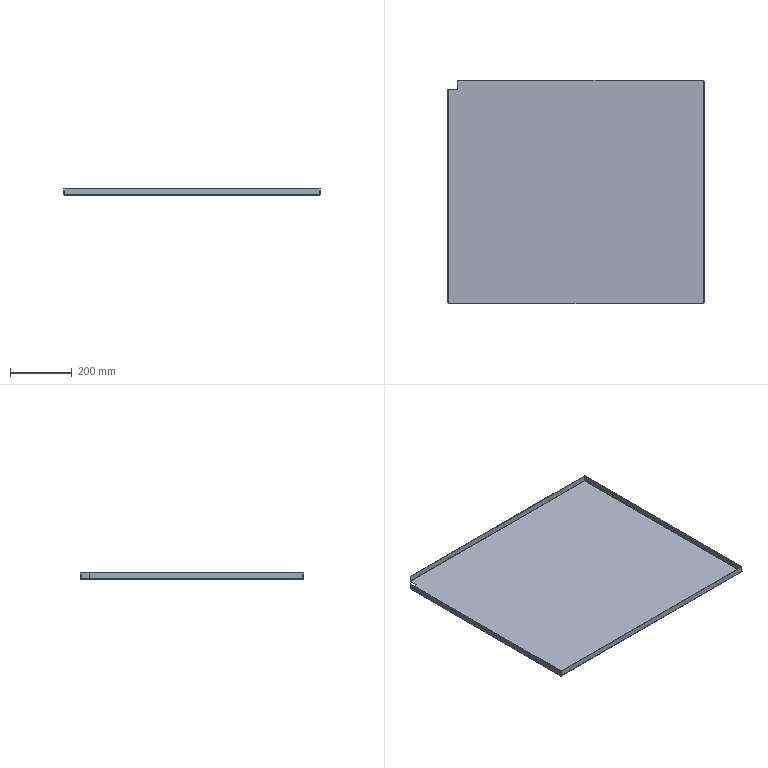Part | SolidWorks | 1 solid | 40 faces | box 830.001 x 723.001 x 20 mm | volume 981196 mm3 | plane 26 | cylinder 8 | spline 6 | commonest cylinder face diameters 0.2 x4 3.2 x4
STEP:
#1=CARTESIAN_POINT('',(-413.5,331.5,18.5));
#2=VERTEX_POINT('',#1);
#3=CARTESIAN_POINT('',(-413.5,331.5,0.1));
#4=VERTEX_POINT('',#3);
#5=CARTESIAN_POINT('',(-413.5,331.5,0.));
#6=DIRECTION('',(0.,0.,-1.));
#7=VECTOR('',#6,1000.);
#8=LINE('',#5,#7);
#9=EDGE_CURVE('',#2,#4,#8,.T.);
#10=ORIENTED_EDGE('',*,*,#9,.T.);
#11=CARTESIAN_POINT('',(-415.,331.5,0.1));
#12=VERTEX_POINT('',#11);
#13=CARTESIAN_POINT('',(-413.5,331.5,0.1));
#14=DIRECTION('',(-1.,0.,0.));
#15=VECTOR('',#14,1000.);
#16=LINE('',#13,#15);
#17=EDGE_CURVE('',#4,#12,#16,.T.);
#18=ORIENTED_EDGE('',*,*,#17,.T.);
#19=CARTESIAN_POINT('',(-415.,331.5,18.5));
#20=VERTEX_POINT('',#19);
#21=CARTESIAN_POINT('',(-415.,331.5,0.));
#22=DIRECTION('',(0.,0.,-1.));
#23=VECTOR('',#22,1000.);
#24=LINE('',#21,#23);
#25=EDGE_CURVE('',#20,#12,#24,.T.);
#26=ORIENTED_EDGE('',*,*,#25,.F.);
#27=CARTESIAN_POINT('',(-434.,331.5,18.5));
#28=DIRECTION('',(1.,0.,0.));
#29=VECTOR('',#28,1000.);
#30=LINE('',#27,#29);
#31=EDGE_CURVE('',#20,#2,#30,.T.);
#32=ORIENTED_EDGE('',*,*,#31,.T.);
#33=EDGE_LOOP('',(#10,#18,#26,#32));
#34=FACE_OUTER_BOUND('',#33,.T.);
#35=CARTESIAN_POINT('',(-434.,331.5,-1.5));
#36=DIRECTION('',(0.,-1.,0.));
#37=DIRECTION('',(0.,0.,-1.));
#38=AXIS2_PLACEMENT_3D('',#35,#36,#37);
#39=PLANE('',#38);
#40=ADVANCED_FACE('',(#34),#39,.F.);
#41=CARTESIAN_POINT('',(-413.4,331.5,-1.5));
#42=VERTEX_POINT('',#41);
#43=CARTESIAN_POINT('',(-384.,331.5,-1.5));
#44=VERTEX_POINT('',#43);
#45=CARTESIAN_POINT('',(-434.,331.5,-1.5));
#46=DIRECTION('',(1.,0.,0.));
#47=VECTOR('',#46,1000.);
#48=LINE('',#45,#47);
#49=EDGE_CURVE('',#42,#44,#48,.T.);
#50=ORIENTED_EDGE('',*,*,#49,.F.);
#51=CARTESIAN_POINT('',(-413.4,331.5,0.));
#52=VERTEX_POINT('',#51);
#53=CARTESIAN_POINT('',(-413.4,331.5,-1.5));
#54=DIRECTION('',(0.,0.,1.));
#55=VECTOR('',#54,1000.);
#56=LINE('',#53,#55);
#57=EDGE_CURVE('',#42,#52,#56,.T.);
#58=ORIENTED_EDGE('',*,*,#57,.T.);
#59=CARTESIAN_POINT('',(-384.,331.5,0.));
#60=VERTEX_POINT('',#59);
#61=CARTESIAN_POINT('',(0.,331.5,0.));
#62=DIRECTION('',(1.,0.,0.));
#63=VECTOR('',#62,1000.);
#64=LINE('',#61,#63);
#65=EDGE_CURVE('',#52,#60,#64,.T.);
#66=ORIENTED_EDGE('',*,*,#65,.T.);
#67=CARTESIAN_POINT('',(-384.,331.5,-1.5));
#68=DIRECTION('',(0.,0.,1.));
#69=VECTOR('',#68,1000.);
#70=LINE('',#67,#69);
#71=EDGE_CURVE('',#44,#60,#70,.T.);
#72=ORIENTED_EDGE('',*,*,#71,.F.);
#73=EDGE_LOOP('',(#50,#58,#66,#72));
#74=FACE_OUTER_BOUND('',#73,.T.);
#75=CARTESIAN_POINT('',(-434.,331.5,-1.5));
#76=DIRECTION('',(0.,-1.,0.));
#77=DIRECTION('',(0.,0.,-1.));
#78=AXIS2_PLACEMENT_3D('',#75,#76,#77);
#79=PLANE('',#78);
#80=ADVANCED_FACE('',(#74),#79,.F.);
#81=CARTESIAN_POINT('',(-384.,359.9,0.));
#82=VERTEX_POINT('',#81);
#83=CARTESIAN_POINT('',(-384.,0.,0.));
#84=DIRECTION('',(0.,1.,0.));
#85=VECTOR('',#84,1000.);
#86=LINE('',#83,#85);
#87=EDGE_CURVE('',#60,#82,#86,.T.);
#88=ORIENTED_EDGE('',*,*,#87,.T.);
#89=CARTESIAN_POINT('',(-384.,359.9,-1.5));
#90=VERTEX_POINT('',#89);
#91=CARTESIAN_POINT('',(-384.,359.9,0.));
#92=DIRECTION('',(0.,0.,-1.));
#93=VECTOR('',#92,1000.);
#94=LINE('',#91,#93);
#95=EDGE_CURVE('',#82,#90,#94,.T.);
#96=ORIENTED_EDGE('',*,*,#95,.T.);
#97=CARTESIAN_POINT('',(-384.,381.5,-1.5));
#98=DIRECTION('',(0.,1.,0.));
#99=VECTOR('',#98,1000.);
#100=LINE('',#97,#99);
#101=EDGE_CURVE('',#44,#90,#100,.T.);
#102=ORIENTED_EDGE('',*,*,#101,.F.);
#103=ORIENTED_EDGE('',*,*,#71,.T.);
#104=EDGE_LOOP('',(#88,#96,#102,#103));
#105=FACE_OUTER_BOUND('',#104,.T.);
#106=CARTESIAN_POINT('',(-384.,381.5,-1.5));
#107=DIRECTION('',(1.,0.,0.));
#108=DIRECTION('',(0.,0.,-1.));
#109=AXIS2_PLACEMENT_3D('',#106,#107,#108);
#110=PLANE('',#109);
#111=ADVANCED_FACE('',(#105),#110,.F.);
#112=CARTESIAN_POINT('',(-384.,361.5,0.1));
#113=VERTEX_POINT('',#112);
#114=CARTESIAN_POINT('',(-384.,361.5,18.5));
#115=VERTEX_POINT('',#114);
#116=CARTESIAN_POINT('',(-384.,361.5,0.));
#117=DIRECTION('',(0.,0.,1.));
#118=VECTOR('',#117,1000.);
#119=LINE('',#116,#118);
#120=EDGE_CURVE('',#113,#115,#119,.T.);
#121=ORIENTED_EDGE('',*,*,#120,.F.);
#122=CARTESIAN_POINT('',(-384.,360.,0.1));
#123=VERTEX_POINT('',#122);
#124=CARTESIAN_POINT('',(-384.,361.5,0.1));
#125=DIRECTION('',(0.,-1.,0.));
#126=VECTOR('',#125,1000.);
#127=LINE('',#124,#126);
#128=EDGE_CURVE('',#113,#123,#127,.T.);
#129=ORIENTED_EDGE('',*,*,#128,.T.);
#130=CARTESIAN_POINT('',(-384.,360.,18.5));
#131=VERTEX_POINT('',#130);
#132=CARTESIAN_POINT('',(-384.,360.,0.));
#133=DIRECTION('',(0.,0.,1.));
#134=VECTOR('',#133,1000.);
#135=LINE('',#132,#134);
#136=EDGE_CURVE('',#123,#131,#135,.T.);
#137=ORIENTED_EDGE('',*,*,#136,.T.);
#138=CARTESIAN_POINT('',(-384.,381.5,18.5));
#139=DIRECTION('',(0.,1.,0.));
#140=VECTOR('',#139,1000.);
#141=LINE('',#138,#140);
#142=EDGE_CURVE('',#131,#115,#141,.T.);
#143=ORIENTED_EDGE('',*,*,#142,.T.);
#144=EDGE_LOOP('',(#121,#129,#137,#143));
#145=FACE_OUTER_BOUND('',#144,.T.);
#146=CARTESIAN_POINT('',(-384.,381.5,-1.5));
#147=DIRECTION('',(1.,0.,0.));
#148=DIRECTION('',(0.,0.,-1.));
#149=AXIS2_PLACEMENT_3D('',#146,#147,#148);
#150=PLANE('',#149);
#151=ADVANCED_FACE('',(#145),#150,.F.);
#152=ORIENTED_EDGE('',*,*,#49,.T.);
#153=ORIENTED_EDGE('',*,*,#101,.T.);
#154=CARTESIAN_POINT('',(413.4,359.9,-1.5));
#155=VERTEX_POINT('',#154);
#156=CARTESIAN_POINT('',(-413.4,359.9,-1.5));
#157=DIRECTION('',(1.,0.,0.));
#158=VECTOR('',#157,1000.);
#159=LINE('',#156,#158);
#160=EDGE_CURVE('',#90,#155,#159,.T.);
#161=ORIENTED_EDGE('',*,*,#160,.T.);
#162=CARTESIAN_POINT('',(413.4,-359.9,-1.5));
#163=VERTEX_POINT('',#162);
#164=CARTESIAN_POINT('',(413.4,359.9,-1.5));
#165=DIRECTION('',(0.,-1.,0.));
#166=VECTOR('',#165,1000.);
#167=LINE('',#164,#166);
#168=EDGE_CURVE('',#155,#163,#167,.T.);
#169=ORIENTED_EDGE('',*,*,#168,.T.);
#170=CARTESIAN_POINT('',(-413.4,-359.9,-1.5));
#171=VERTEX_POINT('',#170);
#172=CARTESIAN_POINT('',(413.4,-359.9,-1.5));
#173=DIRECTION('',(-1.,0.,0.));
#174=VECTOR('',#173,1000.);
#175=LINE('',#172,#174);
#176=EDGE_CURVE('',#163,#171,#175,.T.);
#177=ORIENTED_EDGE('',*,*,#176,.T.);
#178=CARTESIAN_POINT('',(-413.4,-359.9,-1.5));
#179=DIRECTION('',(0.,1.,0.));
#180=VECTOR('',#179,1000.);
#181=LINE('',#178,#180);
#182=EDGE_CURVE('',#171,#42,#181,.T.);
#183=ORIENTED_EDGE('',*,*,#182,.T.);
#184=EDGE_LOOP('',(#152,#153,#161,#169,#177,#183));
#185=FACE_OUTER_BOUND('',#184,.T.);
#186=CARTESIAN_POINT('',(0.,0.,-1.5));
#187=DIRECTION('',(0.,0.,1.));
#188=DIRECTION('',(1.,0.,0.));
#189=AXIS2_PLACEMENT_3D('',#186,#187,#188);
#190=PLANE('',#189);
#191=ADVANCED_FACE('',(#185),#190,.F.);
#192=ORIENTED_EDGE('',*,*,#87,.F.);
#193=ORIENTED_EDGE('',*,*,#65,.F.);
#194=CARTESIAN_POINT('',(-413.4,-359.9,0.));
#195=VERTEX_POINT('',#194);
#196=CARTESIAN_POINT('',(-413.4,-359.9,0.));
#197=DIRECTION('',(0.,1.,0.));
#198=VECTOR('',#197,1000.);
#199=LINE('',#196,#198);
#200=EDGE_CURVE('',#195,#52,#199,.T.);
#201=ORIENTED_EDGE('',*,*,#200,.F.);
#202=CARTESIAN_POINT('',(413.4,-359.9,0.));
#203=VERTEX_POINT('',#202);
#204=CARTESIAN_POINT('',(413.4,-359.9,0.));
#205=DIRECTION('',(-1.,0.,0.));
#206=VECTOR('',#205,1000.);
#207=LINE('',#204,#206);
#208=EDGE_CURVE('',#203,#195,#207,.T.);
#209=ORIENTED_EDGE('',*,*,#208,.F.);
#210=CARTESIAN_POINT('',(413.4,359.9,0.));
#211=VERTEX_POINT('',#210);
#212=CARTESIAN_POINT('',(413.4,359.9,0.));
#213=DIRECTION('',(0.,-1.,0.));
#214=VECTOR('',#213,1000.);
#215=LINE('',#212,#214);
#216=EDGE_CURVE('',#211,#203,#215,.T.);
#217=ORIENTED_EDGE('',*,*,#216,.F.);
#218=CARTESIAN_POINT('',(-413.4,359.9,0.));
#219=DIRECTION('',(1.,0.,0.));
#220=VECTOR('',#219,1000.);
#221=LINE('',#218,#220);
#222=EDGE_CURVE('',#82,#211,#221,.T.);
#223=ORIENTED_EDGE('',*,*,#222,.F.);
#224=EDGE_LOOP('',(#192,#193,#201,#209,#217,#223));
#225=FACE_OUTER_BOUND('',#224,.T.);
#226=CARTESIAN_POINT('',(0.,0.,0.));
#227=DIRECTION('',(0.,0.,1.));
#228=DIRECTION('',(1.,0.,0.));
#229=AXIS2_PLACEMENT_3D('',#226,#227,#228);
#230=PLANE('',#229);
#231=ADVANCED_FACE('',(#225),#230,.T.);
#232=CARTESIAN_POINT('',(-413.5,-359.293,0.1));
#233=VERTEX_POINT('',#232);
#234=CARTESIAN_POINT('',(-413.5,-359.293,0.1));
#235=CARTESIAN_POINT('',(-413.5,-359.394,0.07382));
#236=CARTESIAN_POINT('',(-413.489,-359.495,0.0478));
#237=CARTESIAN_POINT('',(-413.452,-359.698,0.01078));
#238=CARTESIAN_POINT('',(-413.426,-359.799,0.));
#239=CARTESIAN_POINT('',(-413.4,-359.9,0.));
#240=B_SPLINE_CURVE_WITH_KNOTS('',3,(#234,#235,#236,#237,#238,#239),.UNSPECIFIED.,.F.,.F.,(4,2,4),(0.,0.5,1.),.UNSPECIFIED.);
#241=EDGE_CURVE('',#233,#195,#240,.T.);
#242=ORIENTED_EDGE('',*,*,#241,.F.);
#243=CARTESIAN_POINT('',(-415.,-359.293,0.1));
#244=VERTEX_POINT('',#243);
#245=CARTESIAN_POINT('',(-413.5,-359.293,0.1));
#246=DIRECTION('',(1.,0.,0.));
#247=VECTOR('',#246,1000.);
#248=LINE('',#245,#247);
#249=EDGE_CURVE('',#244,#233,#248,.T.);
#250=ORIENTED_EDGE('',*,*,#249,.F.);
#251=CARTESIAN_POINT('',(-415.,-359.293,0.1));
#252=CARTESIAN_POINT('',(-415.,-359.344,-0.1115));
#253=CARTESIAN_POINT('',(-414.96,-359.393,-0.3151));
#254=CARTESIAN_POINT('',(-414.799,-359.495,-0.7048));
#255=CARTESIAN_POINT('',(-414.681,-359.545,-0.881));
#256=CARTESIAN_POINT('',(-414.458,-359.621,-1.105));
#257=CARTESIAN_POINT('',(-414.378,-359.647,-1.171));
#258=CARTESIAN_POINT('',(-414.204,-359.697,-1.287));
#259=CARTESIAN_POINT('',(-414.11,-359.723,-1.338));
#260=CARTESIAN_POINT('',(-413.82,-359.799,-1.458));
#261=CARTESIAN_POINT('',(-413.612,-359.849,-1.5));
#262=CARTESIAN_POINT('',(-413.4,-359.9,-1.5));
#263=B_SPLINE_CURVE_WITH_KNOTS('',3,(#251,#252,#253,#254,#255,#256,#257,#258,#259,#260,#261,#262),.UNSPECIFIED.,.F.,.F.,(4,2,2,2,2,4),(0.,0.0006399,0.00128,0.0016,0.00192,0.00256),.UNSPECIFIED.);
#264=EDGE_CURVE('',#244,#171,#263,.T.);
#265=ORIENTED_EDGE('',*,*,#264,.T.);
#266=CARTESIAN_POINT('',(-413.4,-359.9,0.));
#267=DIRECTION('',(0.,0.,-1.));
#268=VECTOR('',#267,1000.);
#269=LINE('',#266,#268);
#270=EDGE_CURVE('',#195,#171,#269,.T.);
#271=ORIENTED_EDGE('',*,*,#270,.F.);
#272=EDGE_LOOP('',(#242,#250,#265,#271));
#273=FACE_OUTER_BOUND('',#272,.T.);
#274=CARTESIAN_POINT('',(-415.015,-359.293,0.1));
#275=CARTESIAN_POINT('',(-415.015,-359.343,-0.1114));
#276=CARTESIAN_POINT('',(-414.973,-359.394,-0.3227));
#277=CARTESIAN_POINT('',(-414.811,-359.495,-0.7133));
#278=CARTESIAN_POINT('',(-414.691,-359.546,-0.8925));
#279=CARTESIAN_POINT('',(-414.392,-359.647,-1.191));
#280=CARTESIAN_POINT('',(-414.213,-359.698,-1.311));
#281=CARTESIAN_POINT('',(-413.823,-359.799,-1.473));
#282=CARTESIAN_POINT('',(-413.611,-359.849,-1.515));
#283=CARTESIAN_POINT('',(-413.4,-359.9,-1.515));
#284=CARTESIAN_POINT('',(-415.,-359.293,0.1));
#285=CARTESIAN_POINT('',(-415.,-359.343,-0.1095));
#286=CARTESIAN_POINT('',(-414.958,-359.394,-0.3188));
#287=CARTESIAN_POINT('',(-414.798,-359.495,-0.7058));
#288=CARTESIAN_POINT('',(-414.679,-359.546,-0.8833));
#289=CARTESIAN_POINT('',(-414.383,-359.647,-1.179));
#290=CARTESIAN_POINT('',(-414.206,-359.698,-1.298));
#291=CARTESIAN_POINT('',(-413.819,-359.799,-1.458));
#292=CARTESIAN_POINT('',(-413.609,-359.849,-1.5));
#293=CARTESIAN_POINT('',(-413.4,-359.9,-1.5));
#294=CARTESIAN_POINT('',(-413.5,-359.293,0.1));
#295=CARTESIAN_POINT('',(-413.5,-359.343,0.08691));
#296=CARTESIAN_POINT('',(-413.497,-359.394,0.07383));
#297=CARTESIAN_POINT('',(-413.487,-359.495,0.04964));
#298=CARTESIAN_POINT('',(-413.48,-359.546,0.03855));
#299=CARTESIAN_POINT('',(-413.461,-359.647,0.02003));
#300=CARTESIAN_POINT('',(-413.45,-359.698,0.01262));
#301=CARTESIAN_POINT('',(-413.426,-359.799,0.002603));
#302=CARTESIAN_POINT('',(-413.413,-359.849,0.));
#303=CARTESIAN_POINT('',(-413.4,-359.9,0.));
#304=B_SPLINE_SURFACE_WITH_KNOTS('',1,3,((#274,#275,#276,#277,#278,#279,#280,#281,#282,#283),(#284,#285,#286,#287,#288,#289,#290,#291,#292,#293),(#294,#295,#296,#297,#298,#299,#300,#301,#302,#303)),.UNSPECIFIED.,.F.,.F.,.F.,(2,1,2),(4,2,2,2,4),(-0.01,0.,1.),(0.,0.25,0.5,0.75,1.),.UNSPECIFIED.);
#305=ADVANCED_FACE('',(#273),#304,.F.);
#306=CARTESIAN_POINT('',(-413.4,331.5,0.1));
#307=DIRECTION('',(0.,1.,0.));
#308=DIRECTION('',(0.,0.,-1.));
#309=AXIS2_PLACEMENT_3D('',#306,#307,#308);
#310=CIRCLE('',#309,1.6);
#311=EDGE_CURVE('',#42,#12,#310,.T.);
#312=ORIENTED_EDGE('',*,*,#311,.F.);
#313=ORIENTED_EDGE('',*,*,#182,.F.);
#314=ORIENTED_EDGE('',*,*,#264,.F.);
#315=CARTESIAN_POINT('',(-415.,361.5,0.1));
#316=DIRECTION('',(0.,1.,0.));
#317=VECTOR('',#316,1000.);
#318=LINE('',#315,#317);
#319=EDGE_CURVE('',#244,#12,#318,.T.);
#320=ORIENTED_EDGE('',*,*,#319,.T.);
#321=EDGE_LOOP('',(#312,#313,#314,#320));
#322=FACE_OUTER_BOUND('',#321,.T.);
#323=CARTESIAN_POINT('',(-413.4,-359.9,0.1));
#324=DIRECTION('',(0.,-1.,0.));
#325=DIRECTION('',(-1.,0.,0.));
#326=AXIS2_PLACEMENT_3D('',#323,#324,#325);
#327=CYLINDRICAL_SURFACE('',#326,1.6);
#328=ADVANCED_FACE('',(#322),#327,.T.);
#329=ORIENTED_EDGE('',*,*,#200,.T.);
#330=CARTESIAN_POINT('',(-413.4,331.5,0.1));
#331=DIRECTION('',(0.,1.,0.));
#332=DIRECTION('',(0.,0.,-1.));
#333=AXIS2_PLACEMENT_3D('',#330,#331,#332);
#334=CIRCLE('',#333,0.1);
#335=EDGE_CURVE('',#52,#4,#334,.T.);
#336=ORIENTED_EDGE('',*,*,#335,.T.);
#337=CARTESIAN_POINT('',(-413.5,361.5,0.1));
#338=DIRECTION('',(0.,-1.,0.));
#339=VECTOR('',#338,1000.);
#340=LINE('',#337,#339);
#341=EDGE_CURVE('',#4,#233,#340,.T.);
#342=ORIENTED_EDGE('',*,*,#341,.T.);
#343=ORIENTED_EDGE('',*,*,#241,.T.);
#344=EDGE_LOOP('',(#329,#336,#342,#343));
#345=FACE_OUTER_BOUND('',#344,.T.);
#346=CARTESIAN_POINT('',(-413.4,-359.9,0.1));
#347=DIRECTION('',(0.,-1.,0.));
#348=DIRECTION('',(-1.,0.,0.));
#349=AXIS2_PLACEMENT_3D('',#346,#347,#348);
#350=CYLINDRICAL_SURFACE('',#349,0.1);
#351=ADVANCED_FACE('',(#345),#350,.F.);
#352=CARTESIAN_POINT('',(-415.,-359.293,18.5));
#353=VERTEX_POINT('',#352);
#354=CARTESIAN_POINT('',(-415.,0.,18.5));
#355=DIRECTION('',(0.,1.,0.));
#356=VECTOR('',#355,1000.);
#357=LINE('',#354,#356);
#358=EDGE_CURVE('',#353,#20,#357,.T.);
#359=ORIENTED_EDGE('',*,*,#358,.T.);
#360=ORIENTED_EDGE('',*,*,#25,.T.);
#361=ORIENTED_EDGE('',*,*,#319,.F.);
#362=CARTESIAN_POINT('',(-415.,-359.293,0.));
#363=DIRECTION('',(0.,0.,1.));
#364=VECTOR('',#363,1000.);
#365=LINE('',#362,#364);
#366=EDGE_CURVE('',#244,#353,#365,.T.);
#367=ORIENTED_EDGE('',*,*,#366,.T.);
#368=EDGE_LOOP('',(#359,#360,#361,#367));
#369=FACE_OUTER_BOUND('',#368,.T.);
#370=CARTESIAN_POINT('',(-415.,0.,0.));
#371=DIRECTION('',(1.,0.,0.));
#372=DIRECTION('',(0.,0.,-1.));
#373=AXIS2_PLACEMENT_3D('',#370,#371,#372);
#374=PLANE('',#373);
#375=ADVANCED_FACE('',(#369),#374,.F.);
#376=ORIENTED_EDGE('',*,*,#9,.F.);
#377=CARTESIAN_POINT('',(-413.5,-359.293,18.5));
#378=VERTEX_POINT('',#377);
#379=CARTESIAN_POINT('',(-413.5,361.5,18.5));
#380=DIRECTION('',(0.,1.,0.));
#381=VECTOR('',#380,1000.);
#382=LINE('',#379,#381);
#383=EDGE_CURVE('',#378,#2,#382,.T.);
#384=ORIENTED_EDGE('',*,*,#383,.F.);
#385=CARTESIAN_POINT('',(-413.5,-359.293,0.));
#386=DIRECTION('',(0.,0.,1.));
#387=VECTOR('',#386,1000.);
#388=LINE('',#385,#387);
#389=EDGE_CURVE('',#233,#378,#388,.T.);
#390=ORIENTED_EDGE('',*,*,#389,.F.);
#391=ORIENTED_EDGE('',*,*,#341,.F.);
#392=EDGE_LOOP('',(#376,#384,#390,#391));
#393=FACE_OUTER_BOUND('',#392,.T.);
#394=CARTESIAN_POINT('',(-413.5,0.,0.));
#395=DIRECTION('',(1.,0.,0.));
#396=DIRECTION('',(0.,0.,-1.));
#397=AXIS2_PLACEMENT_3D('',#394,#395,#396);
#398=PLANE('',#397);
#399=ADVANCED_FACE('',(#393),#398,.T.);
#400=ORIENTED_EDGE('',*,*,#383,.T.);
#401=ORIENTED_EDGE('',*,*,#31,.F.);
#402=ORIENTED_EDGE('',*,*,#358,.F.);
#403=CARTESIAN_POINT('',(-415.,-359.293,18.5));
#404=DIRECTION('',(1.,0.,0.));
#405=VECTOR('',#404,1000.);
#406=LINE('',#403,#405);
#407=EDGE_CURVE('',#353,#378,#406,.T.);
#408=ORIENTED_EDGE('',*,*,#407,.T.);
#409=EDGE_LOOP('',(#400,#401,#402,#408));
#410=FACE_OUTER_BOUND('',#409,.T.);
#411=CARTESIAN_POINT('',(-415.,361.5,18.5));
#412=DIRECTION('',(0.,0.,-1.));
#413=DIRECTION('',(-1.,0.,0.));
#414=AXIS2_PLACEMENT_3D('',#411,#412,#413);
#415=PLANE('',#414);
#416=ADVANCED_FACE('',(#410),#415,.F.);
#417=ORIENTED_EDGE('',*,*,#407,.F.);
#418=ORIENTED_EDGE('',*,*,#366,.F.);
#419=ORIENTED_EDGE('',*,*,#249,.T.);
#420=ORIENTED_EDGE('',*,*,#389,.T.);
#421=EDGE_LOOP('',(#417,#418,#419,#420));
#422=FACE_OUTER_BOUND('',#421,.T.);
#423=CARTESIAN_POINT('',(-413.5,-359.293,0.));
#424=DIRECTION('',(0.,1.,0.));
#425=DIRECTION('',(0.,0.,1.));
#426=AXIS2_PLACEMENT_3D('',#423,#424,#425);
#427=PLANE('',#426);
#428=ADVANCED_FACE('',(#422),#427,.F.);
#429=CARTESIAN_POINT('',(412.793,361.5,0.1));
#430=VERTEX_POINT('',#429);
#431=CARTESIAN_POINT('',(412.793,360.,0.1));
#432=VERTEX_POINT('',#431);
#433=CARTESIAN_POINT('',(412.793,360.,0.1));
#434=DIRECTION('',(0.,-1.,0.));
#435=VECTOR('',#434,1000.);
#436=LINE('',#433,#435);
#437=EDGE_CURVE('',#430,#432,#436,.T.);
#438=ORIENTED_EDGE('',*,*,#437,.T.);
#439=CARTESIAN_POINT('',(413.4,359.9,0.));
#440=CARTESIAN_POINT('',(413.299,359.926,0.));
#441=CARTESIAN_POINT('',(413.198,359.952,0.01078));
#442=CARTESIAN_POINT('',(412.995,359.989,0.0478));
#443=CARTESIAN_POINT('',(412.894,360.,0.07382));
#444=CARTESIAN_POINT('',(412.793,360.,0.1));
#445=B_SPLINE_CURVE_WITH_KNOTS('',3,(#439,#440,#441,#442,#443,#444),.UNSPECIFIED.,.F.,.F.,(4,2,4),(0.,0.5,1.),.UNSPECIFIED.);
#446=EDGE_CURVE('',#211,#432,#445,.T.);
#447=ORIENTED_EDGE('',*,*,#446,.F.);
#448=CARTESIAN_POINT('',(413.4,359.9,0.));
#449=DIRECTION('',(0.,0.,-1.));
#450=VECTOR('',#449,1000.);
#451=LINE('',#448,#450);
#452=EDGE_CURVE('',#211,#155,#451,.T.);
#453=ORIENTED_EDGE('',*,*,#452,.T.);
#454=CARTESIAN_POINT('',(413.4,359.9,-1.5));
#455=CARTESIAN_POINT('',(413.349,360.112,-1.5));
#456=CARTESIAN_POINT('',(413.3,360.315,-1.46));
#457=CARTESIAN_POINT('',(413.198,360.705,-1.299));
#458=CARTESIAN_POINT('',(413.148,360.881,-1.181));
#459=CARTESIAN_POINT('',(413.071,361.105,-0.9582));
#460=CARTESIAN_POINT('',(413.046,361.171,-0.8775));
#461=CARTESIAN_POINT('',(412.996,361.287,-0.7041));
#462=CARTESIAN_POINT('',(412.97,361.338,-0.6103));
#463=CARTESIAN_POINT('',(412.894,361.458,-0.32));
#464=CARTESIAN_POINT('',(412.844,361.5,-0.1115));
#465=CARTESIAN_POINT('',(412.793,361.5,0.1));
#466=B_SPLINE_CURVE_WITH_KNOTS('',3,(#454,#455,#456,#457,#458,#459,#460,#461,#462,#463,#464,#465),.UNSPECIFIED.,.F.,.F.,(4,2,2,2,2,4),(0.,0.0006399,0.00128,0.0016,0.00192,0.00256),.UNSPECIFIED.);
#467=EDGE_CURVE('',#155,#430,#466,.T.);
#468=ORIENTED_EDGE('',*,*,#467,.T.);
#469=EDGE_LOOP('',(#438,#447,#453,#468));
#470=FACE_OUTER_BOUND('',#469,.T.);
#471=CARTESIAN_POINT('',(413.4,359.9,-1.515));
#472=CARTESIAN_POINT('',(413.349,360.111,-1.515));
#473=CARTESIAN_POINT('',(413.299,360.323,-1.473));
#474=CARTESIAN_POINT('',(413.198,360.713,-1.311));
#475=CARTESIAN_POINT('',(413.147,360.892,-1.191));
#476=CARTESIAN_POINT('',(413.046,361.191,-0.8925));
#477=CARTESIAN_POINT('',(412.995,361.311,-0.7133));
#478=CARTESIAN_POINT('',(412.894,361.473,-0.3227));
#479=CARTESIAN_POINT('',(412.843,361.515,-0.1114));
#480=CARTESIAN_POINT('',(412.793,361.515,0.1));
#481=CARTESIAN_POINT('',(413.4,359.9,-1.5));
#482=CARTESIAN_POINT('',(413.349,360.109,-1.5));
#483=CARTESIAN_POINT('',(413.299,360.319,-1.458));
#484=CARTESIAN_POINT('',(413.198,360.706,-1.298));
#485=CARTESIAN_POINT('',(413.147,360.883,-1.179));
#486=CARTESIAN_POINT('',(413.046,361.179,-0.8833));
#487=CARTESIAN_POINT('',(412.995,361.298,-0.7058));
#488=CARTESIAN_POINT('',(412.894,361.458,-0.3188));
#489=CARTESIAN_POINT('',(412.843,361.5,-0.1095));
#490=CARTESIAN_POINT('',(412.793,361.5,0.1));
#491=CARTESIAN_POINT('',(413.4,359.9,0.));
#492=CARTESIAN_POINT('',(413.349,359.913,0.));
#493=CARTESIAN_POINT('',(413.299,359.926,0.002603));
#494=CARTESIAN_POINT('',(413.198,359.95,0.01262));
#495=CARTESIAN_POINT('',(413.147,359.961,0.02003));
#496=CARTESIAN_POINT('',(413.046,359.98,0.03855));
#497=CARTESIAN_POINT('',(412.995,359.987,0.04964));
#498=CARTESIAN_POINT('',(412.894,359.997,0.07383));
#499=CARTESIAN_POINT('',(412.843,360.,0.08691));
#500=CARTESIAN_POINT('',(412.793,360.,0.1));
#501=B_SPLINE_SURFACE_WITH_KNOTS('',1,3,((#471,#472,#473,#474,#475,#476,#477,#478,#479,#480),(#481,#482,#483,#484,#485,#486,#487,#488,#489,#490),(#491,#492,#493,#494,#495,#496,#497,#498,#499,#500)),.UNSPECIFIED.,.F.,.F.,.F.,(2,1,2),(4,2,2,2,4),(-0.01,0.,1.),(0.,0.25,0.5,0.75,1.),.UNSPECIFIED.);
#502=ADVANCED_FACE('',(#470),#501,.F.);
#503=CARTESIAN_POINT('',(-384.,359.9,0.1));
#504=DIRECTION('',(-1.,0.,0.));
#505=DIRECTION('',(0.,0.,-1.));
#506=AXIS2_PLACEMENT_3D('',#503,#504,#505);
#507=CIRCLE('',#506,1.6);
#508=EDGE_CURVE('',#113,#90,#507,.T.);
#509=ORIENTED_EDGE('',*,*,#508,.F.);
#510=CARTESIAN_POINT('',(415.,361.5,0.1));
#511=DIRECTION('',(1.,0.,0.));
#512=VECTOR('',#511,1000.);
#513=LINE('',#510,#512);
#514=EDGE_CURVE('',#113,#430,#513,.T.);
#515=ORIENTED_EDGE('',*,*,#514,.T.);
#516=ORIENTED_EDGE('',*,*,#467,.F.);
#517=ORIENTED_EDGE('',*,*,#160,.F.);
#518=EDGE_LOOP('',(#509,#515,#516,#517));
#519=FACE_OUTER_BOUND('',#518,.T.);
#520=CARTESIAN_POINT('',(-413.4,359.9,0.1));
#521=DIRECTION('',(-1.,0.,0.));
#522=DIRECTION('',(0.,1.,0.));
#523=AXIS2_PLACEMENT_3D('',#520,#521,#522);
#524=CYLINDRICAL_SURFACE('',#523,1.6);
#525=ADVANCED_FACE('',(#519),#524,.T.);
#526=CARTESIAN_POINT('',(415.,360.,0.1));
#527=DIRECTION('',(-1.,0.,0.));
#528=VECTOR('',#527,1000.);
#529=LINE('',#526,#528);
#530=EDGE_CURVE('',#432,#123,#529,.T.);
#531=ORIENTED_EDGE('',*,*,#530,.T.);
#532=CARTESIAN_POINT('',(-384.,359.9,0.1));
#533=DIRECTION('',(-1.,0.,0.));
#534=DIRECTION('',(0.,0.,-1.));
#535=AXIS2_PLACEMENT_3D('',#532,#533,#534);
#536=CIRCLE('',#535,0.1);
#537=EDGE_CURVE('',#123,#82,#536,.T.);
#538=ORIENTED_EDGE('',*,*,#537,.T.);
#539=ORIENTED_EDGE('',*,*,#222,.T.);
#540=ORIENTED_EDGE('',*,*,#446,.T.);
#541=EDGE_LOOP('',(#531,#538,#539,#540));
#542=FACE_OUTER_BOUND('',#541,.T.);
#543=CARTESIAN_POINT('',(-413.4,359.9,0.1));
#544=DIRECTION('',(-1.,0.,0.));
#545=DIRECTION('',(0.,1.,0.));
#546=AXIS2_PLACEMENT_3D('',#543,#544,#545);
#547=CYLINDRICAL_SURFACE('',#546,0.1);
#548=ADVANCED_FACE('',(#542),#547,.F.);
#549=CARTESIAN_POINT('',(412.793,361.5,18.5));
#550=VERTEX_POINT('',#549);
#551=CARTESIAN_POINT('',(412.793,361.5,0.));
#552=DIRECTION('',(0.,0.,1.));
#553=VECTOR('',#552,1000.);
#554=LINE('',#551,#553);
#555=EDGE_CURVE('',#430,#550,#554,.T.);
#556=ORIENTED_EDGE('',*,*,#555,.T.);
#557=CARTESIAN_POINT('',(412.793,360.,18.5));
#558=VERTEX_POINT('',#557);
#559=CARTESIAN_POINT('',(412.793,360.,18.5));
#560=DIRECTION('',(0.,-1.,0.));
#561=VECTOR('',#560,1000.);
#562=LINE('',#559,#561);
#563=EDGE_CURVE('',#550,#558,#562,.T.);
#564=ORIENTED_EDGE('',*,*,#563,.T.);
#565=CARTESIAN_POINT('',(412.793,360.,0.));
#566=DIRECTION('',(0.,0.,1.));
#567=VECTOR('',#566,1000.);
#568=LINE('',#565,#567);
#569=EDGE_CURVE('',#432,#558,#568,.T.);
#570=ORIENTED_EDGE('',*,*,#569,.F.);
#571=ORIENTED_EDGE('',*,*,#437,.F.);
#572=EDGE_LOOP('',(#556,#564,#570,#571));
#573=FACE_OUTER_BOUND('',#572,.T.);
#574=CARTESIAN_POINT('',(412.793,360.,0.));
#575=DIRECTION('',(1.,0.,0.));
#576=DIRECTION('',(0.,0.,-1.));
#577=AXIS2_PLACEMENT_3D('',#574,#575,#576);
#578=PLANE('',#577);
#579=ADVANCED_FACE('',(#573),#578,.T.);
#580=ORIENTED_EDGE('',*,*,#514,.F.);
#581=ORIENTED_EDGE('',*,*,#120,.T.);
#582=CARTESIAN_POINT('',(0.,361.5,18.5));
#583=DIRECTION('',(1.,0.,0.));
#584=VECTOR('',#583,1000.);
#585=LINE('',#582,#584);
#586=EDGE_CURVE('',#115,#550,#585,.T.);
#587=ORIENTED_EDGE('',*,*,#586,.T.);
#588=ORIENTED_EDGE('',*,*,#555,.F.);
#589=EDGE_LOOP('',(#580,#581,#587,#588));
#590=FACE_OUTER_BOUND('',#589,.T.);
#591=CARTESIAN_POINT('',(0.,361.5,0.));
#592=DIRECTION('',(0.,-1.,0.));
#593=DIRECTION('',(0.,0.,-1.));
#594=AXIS2_PLACEMENT_3D('',#591,#592,#593);
#595=PLANE('',#594);
#596=ADVANCED_FACE('',(#590),#595,.F.);
#597=ORIENTED_EDGE('',*,*,#136,.F.);
#598=ORIENTED_EDGE('',*,*,#530,.F.);
#599=ORIENTED_EDGE('',*,*,#569,.T.);
#600=CARTESIAN_POINT('',(415.,360.,18.5));
#601=DIRECTION('',(1.,0.,0.));
#602=VECTOR('',#601,1000.);
#603=LINE('',#600,#602);
#604=EDGE_CURVE('',#131,#558,#603,.T.);
#605=ORIENTED_EDGE('',*,*,#604,.F.);
#606=EDGE_LOOP('',(#597,#598,#599,#605));
#607=FACE_OUTER_BOUND('',#606,.T.);
#608=CARTESIAN_POINT('',(0.,360.,0.));
#609=DIRECTION('',(0.,-1.,0.));
#610=DIRECTION('',(0.,0.,-1.));
#611=AXIS2_PLACEMENT_3D('',#608,#609,#610);
#612=PLANE('',#611);
#613=ADVANCED_FACE('',(#607),#612,.T.);
#614=ORIENTED_EDGE('',*,*,#586,.F.);
#615=ORIENTED_EDGE('',*,*,#142,.F.);
#616=ORIENTED_EDGE('',*,*,#604,.T.);
#617=ORIENTED_EDGE('',*,*,#563,.F.);
#618=EDGE_LOOP('',(#614,#615,#616,#617));
#619=FACE_OUTER_BOUND('',#618,.T.);
#620=CARTESIAN_POINT('',(415.,361.5,18.5));
#621=DIRECTION('',(0.,0.,-1.));
#622=DIRECTION('',(0.,1.,0.));
#623=AXIS2_PLACEMENT_3D('',#620,#621,#622);
#624=PLANE('',#623);
#625=ADVANCED_FACE('',(#619),#624,.F.);
#626=CARTESIAN_POINT('',(415.,-359.293,0.1));
#627=VERTEX_POINT('',#626);
#628=CARTESIAN_POINT('',(413.5,-359.293,0.1));
#629=VERTEX_POINT('',#628);
#630=CARTESIAN_POINT('',(413.5,-359.293,0.1));
#631=DIRECTION('',(-1.,0.,0.));
#632=VECTOR('',#631,1000.);
#633=LINE('',#630,#632);
#634=EDGE_CURVE('',#627,#629,#633,.T.);
#635=ORIENTED_EDGE('',*,*,#634,.T.);
#636=CARTESIAN_POINT('',(413.4,-359.9,0.));
#637=CARTESIAN_POINT('',(413.426,-359.799,0.));
#638=CARTESIAN_POINT('',(413.452,-359.698,0.01078));
#639=CARTESIAN_POINT('',(413.489,-359.495,0.0478));
#640=CARTESIAN_POINT('',(413.5,-359.394,0.07382));
#641=CARTESIAN_POINT('',(413.5,-359.293,0.1));
#642=B_SPLINE_CURVE_WITH_KNOTS('',3,(#636,#637,#638,#639,#640,#641),.UNSPECIFIED.,.F.,.F.,(4,2,4),(0.,0.5,1.),.UNSPECIFIED.);
#643=EDGE_CURVE('',#203,#629,#642,.T.);
#644=ORIENTED_EDGE('',*,*,#643,.F.);
#645=CARTESIAN_POINT('',(413.4,-359.9,0.));
#646=DIRECTION('',(0.,0.,-1.));
#647=VECTOR('',#646,1000.);
#648=LINE('',#645,#647);
#649=EDGE_CURVE('',#203,#163,#648,.T.);
#650=ORIENTED_EDGE('',*,*,#649,.T.);
#651=CARTESIAN_POINT('',(413.4,-359.9,-1.5));
#652=CARTESIAN_POINT('',(413.612,-359.849,-1.5));
#653=CARTESIAN_POINT('',(413.815,-359.8,-1.46));
#654=CARTESIAN_POINT('',(414.205,-359.698,-1.299));
#655=CARTESIAN_POINT('',(414.381,-359.648,-1.181));
#656=CARTESIAN_POINT('',(414.605,-359.571,-0.9582));
#657=CARTESIAN_POINT('',(414.671,-359.546,-0.8775));
#658=CARTESIAN_POINT('',(414.787,-359.496,-0.7041));
#659=CARTESIAN_POINT('',(414.838,-359.47,-0.6103));
#660=CARTESIAN_POINT('',(414.958,-359.394,-0.32));
#661=CARTESIAN_POINT('',(415.,-359.344,-0.1115));
#662=CARTESIAN_POINT('',(415.,-359.293,0.1));
#663=B_SPLINE_CURVE_WITH_KNOTS('',3,(#651,#652,#653,#654,#655,#656,#657,#658,#659,#660,#661,#662),.UNSPECIFIED.,.F.,.F.,(4,2,2,2,2,4),(0.,0.0006399,0.00128,0.0016,0.00192,0.00256),.UNSPECIFIED.);
#664=EDGE_CURVE('',#163,#627,#663,.T.);
#665=ORIENTED_EDGE('',*,*,#664,.T.);
#666=EDGE_LOOP('',(#635,#644,#650,#665));
#667=FACE_OUTER_BOUND('',#666,.T.);
#668=CARTESIAN_POINT('',(413.4,-359.9,-1.515));
#669=CARTESIAN_POINT('',(413.611,-359.849,-1.515));
#670=CARTESIAN_POINT('',(413.823,-359.799,-1.473));
#671=CARTESIAN_POINT('',(414.213,-359.698,-1.311));
#672=CARTESIAN_POINT('',(414.392,-359.647,-1.191));
#673=CARTESIAN_POINT('',(414.691,-359.546,-0.8925));
#674=CARTESIAN_POINT('',(414.811,-359.495,-0.7133));
#675=CARTESIAN_POINT('',(414.973,-359.394,-0.3227));
#676=CARTESIAN_POINT('',(415.015,-359.343,-0.1114));
#677=CARTESIAN_POINT('',(415.015,-359.293,0.1));
#678=CARTESIAN_POINT('',(413.4,-359.9,-1.5));
#679=CARTESIAN_POINT('',(413.609,-359.849,-1.5));
#680=CARTESIAN_POINT('',(413.819,-359.799,-1.458));
#681=CARTESIAN_POINT('',(414.206,-359.698,-1.298));
#682=CARTESIAN_POINT('',(414.383,-359.647,-1.179));
#683=CARTESIAN_POINT('',(414.679,-359.546,-0.8833));
#684=CARTESIAN_POINT('',(414.798,-359.495,-0.7058));
#685=CARTESIAN_POINT('',(414.958,-359.394,-0.3188));
#686=CARTESIAN_POINT('',(415.,-359.343,-0.1095));
#687=CARTESIAN_POINT('',(415.,-359.293,0.1));
#688=CARTESIAN_POINT('',(413.4,-359.9,0.));
#689=CARTESIAN_POINT('',(413.413,-359.849,0.));
#690=CARTESIAN_POINT('',(413.426,-359.799,0.002603));
#691=CARTESIAN_POINT('',(413.45,-359.698,0.01262));
#692=CARTESIAN_POINT('',(413.461,-359.647,0.02003));
#693=CARTESIAN_POINT('',(413.48,-359.546,0.03855));
#694=CARTESIAN_POINT('',(413.487,-359.495,0.04964));
#695=CARTESIAN_POINT('',(413.497,-359.394,0.07383));
#696=CARTESIAN_POINT('',(413.5,-359.343,0.08691));
#697=CARTESIAN_POINT('',(413.5,-359.293,0.1));
#698=B_SPLINE_SURFACE_WITH_KNOTS('',1,3,((#668,#669,#670,#671,#672,#673,#674,#675,#676,#677),(#678,#679,#680,#681,#682,#683,#684,#685,#686,#687),(#688,#689,#690,#691,#692,#693,#694,#695,#696,#697)),.UNSPECIFIED.,.F.,.F.,.F.,(2,1,2),(4,2,2,2,4),(-0.01,0.,1.),(0.,0.25,0.5,0.75,1.),.UNSPECIFIED.);
#699=ADVANCED_FACE('',(#667),#698,.F.);
#700=CARTESIAN_POINT('',(413.5,359.293,0.1));
#701=VERTEX_POINT('',#700);
#702=CARTESIAN_POINT('',(413.5,359.293,0.1));
#703=CARTESIAN_POINT('',(413.5,359.394,0.07382));
#704=CARTESIAN_POINT('',(413.489,359.495,0.0478));
#705=CARTESIAN_POINT('',(413.452,359.698,0.01078));
#706=CARTESIAN_POINT('',(413.426,359.799,0.));
#707=CARTESIAN_POINT('',(413.4,359.9,0.));
#708=B_SPLINE_CURVE_WITH_KNOTS('',3,(#702,#703,#704,#705,#706,#707),.UNSPECIFIED.,.F.,.F.,(4,2,4),(0.,0.5,1.),.UNSPECIFIED.);
#709=EDGE_CURVE('',#701,#211,#708,.T.);
#710=ORIENTED_EDGE('',*,*,#709,.F.);
#711=CARTESIAN_POINT('',(415.,359.293,0.1));
#712=VERTEX_POINT('',#711);
#713=CARTESIAN_POINT('',(413.5,359.293,0.1));
#714=DIRECTION('',(-1.,0.,0.));
#715=VECTOR('',#714,1000.);
#716=LINE('',#713,#715);
#717=EDGE_CURVE('',#712,#701,#716,.T.);
#718=ORIENTED_EDGE('',*,*,#717,.F.);
#719=CARTESIAN_POINT('',(415.,359.293,0.1));
#720=CARTESIAN_POINT('',(415.,359.344,-0.1115));
#721=CARTESIAN_POINT('',(414.96,359.393,-0.3151));
#722=CARTESIAN_POINT('',(414.799,359.495,-0.7048));
#723=CARTESIAN_POINT('',(414.681,359.545,-0.881));
#724=CARTESIAN_POINT('',(414.458,359.621,-1.105));
#725=CARTESIAN_POINT('',(414.378,359.647,-1.171));
#726=CARTESIAN_POINT('',(414.204,359.697,-1.287));
#727=CARTESIAN_POINT('',(414.11,359.723,-1.338));
#728=CARTESIAN_POINT('',(413.82,359.799,-1.458));
#729=CARTESIAN_POINT('',(413.612,359.849,-1.5));
#730=CARTESIAN_POINT('',(413.4,359.9,-1.5));
#731=B_SPLINE_CURVE_WITH_KNOTS('',3,(#719,#720,#721,#722,#723,#724,#725,#726,#727,#728,#729,#730),.UNSPECIFIED.,.F.,.F.,(4,2,2,2,2,4),(0.,0.0006399,0.00128,0.0016,0.00192,0.00256),.UNSPECIFIED.);
#732=EDGE_CURVE('',#712,#155,#731,.T.);
#733=ORIENTED_EDGE('',*,*,#732,.T.);
#734=ORIENTED_EDGE('',*,*,#452,.F.);
#735=EDGE_LOOP('',(#710,#718,#733,#734));
#736=FACE_OUTER_BOUND('',#735,.T.);
#737=CARTESIAN_POINT('',(415.015,359.293,0.1));
#738=CARTESIAN_POINT('',(415.015,359.343,-0.1114));
#739=CARTESIAN_POINT('',(414.973,359.394,-0.3227));
#740=CARTESIAN_POINT('',(414.811,359.495,-0.7133));
#741=CARTESIAN_POINT('',(414.691,359.546,-0.8925));
#742=CARTESIAN_POINT('',(414.392,359.647,-1.191));
#743=CARTESIAN_POINT('',(414.213,359.698,-1.311));
#744=CARTESIAN_POINT('',(413.823,359.799,-1.473));
#745=CARTESIAN_POINT('',(413.611,359.849,-1.515));
#746=CARTESIAN_POINT('',(413.4,359.9,-1.515));
#747=CARTESIAN_POINT('',(415.,359.293,0.1));
#748=CARTESIAN_POINT('',(415.,359.343,-0.1095));
#749=CARTESIAN_POINT('',(414.958,359.394,-0.3188));
#750=CARTESIAN_POINT('',(414.798,359.495,-0.7058));
#751=CARTESIAN_POINT('',(414.679,359.546,-0.8833));
#752=CARTESIAN_POINT('',(414.383,359.647,-1.179));
#753=CARTESIAN_POINT('',(414.206,359.698,-1.298));
#754=CARTESIAN_POINT('',(413.819,359.799,-1.458));
#755=CARTESIAN_POINT('',(413.609,359.849,-1.5));
#756=CARTESIAN_POINT('',(413.4,359.9,-1.5));
#757=CARTESIAN_POINT('',(413.5,359.293,0.1));
#758=CARTESIAN_POINT('',(413.5,359.343,0.08691));
#759=CARTESIAN_POINT('',(413.497,359.394,0.07383));
#760=CARTESIAN_POINT('',(413.487,359.495,0.04964));
#761=CARTESIAN_POINT('',(413.48,359.546,0.03855));
#762=CARTESIAN_POINT('',(413.461,359.647,0.02003));
#763=CARTESIAN_POINT('',(413.45,359.698,0.01262));
#764=CARTESIAN_POINT('',(413.426,359.799,0.002603));
#765=CARTESIAN_POINT('',(413.413,359.849,0.));
#766=CARTESIAN_POINT('',(413.4,359.9,0.));
#767=B_SPLINE_SURFACE_WITH_KNOTS('',1,3,((#737,#738,#739,#740,#741,#742,#743,#744,#745,#746),(#747,#748,#749,#750,#751,#752,#753,#754,#755,#756),(#757,#758,#759,#760,#761,#762,#763,#764,#765,#766)),.UNSPECIFIED.,.F.,.F.,.F.,(2,1,2),(4,2,2,2,4),(-0.01,0.,1.),(0.,0.25,0.5,0.75,1.),.UNSPECIFIED.);
#768=ADVANCED_FACE('',(#736),#767,.F.);
#769=ORIENTED_EDGE('',*,*,#168,.F.);
#770=ORIENTED_EDGE('',*,*,#732,.F.);
#771=CARTESIAN_POINT('',(415.,-361.5,0.1));
#772=DIRECTION('',(0.,-1.,0.));
#773=VECTOR('',#772,1000.);
#774=LINE('',#771,#773);
#775=EDGE_CURVE('',#712,#627,#774,.T.);
#776=ORIENTED_EDGE('',*,*,#775,.T.);
#777=ORIENTED_EDGE('',*,*,#664,.F.);
#778=EDGE_LOOP('',(#769,#770,#776,#777));
#779=FACE_OUTER_BOUND('',#778,.T.);
#780=CARTESIAN_POINT('',(413.4,359.9,0.1));
#781=DIRECTION('',(0.,1.,0.));
#782=DIRECTION('',(1.,0.,0.));
#783=AXIS2_PLACEMENT_3D('',#780,#781,#782);
#784=CYLINDRICAL_SURFACE('',#783,1.6);
#785=ADVANCED_FACE('',(#779),#784,.T.);
#786=ORIENTED_EDGE('',*,*,#216,.T.);
#787=ORIENTED_EDGE('',*,*,#643,.T.);
#788=CARTESIAN_POINT('',(413.5,-361.5,0.1));
#789=DIRECTION('',(0.,1.,0.));
#790=VECTOR('',#789,1000.);
#791=LINE('',#788,#790);
#792=EDGE_CURVE('',#629,#701,#791,.T.);
#793=ORIENTED_EDGE('',*,*,#792,.T.);
#794=ORIENTED_EDGE('',*,*,#709,.T.);
#795=EDGE_LOOP('',(#786,#787,#793,#794));
#796=FACE_OUTER_BOUND('',#795,.T.);
#797=CARTESIAN_POINT('',(413.4,359.9,0.1));
#798=DIRECTION('',(0.,1.,0.));
#799=DIRECTION('',(1.,0.,0.));
#800=AXIS2_PLACEMENT_3D('',#797,#798,#799);
#801=CYLINDRICAL_SURFACE('',#800,0.1);
#802=ADVANCED_FACE('',(#796),#801,.F.);
#803=CARTESIAN_POINT('',(415.,-359.293,18.5));
#804=VERTEX_POINT('',#803);
#805=CARTESIAN_POINT('',(415.,-359.293,0.));
#806=DIRECTION('',(0.,0.,1.));
#807=VECTOR('',#806,1000.);
#808=LINE('',#805,#807);
#809=EDGE_CURVE('',#627,#804,#808,.T.);
#810=ORIENTED_EDGE('',*,*,#809,.T.);
#811=CARTESIAN_POINT('',(413.5,-359.293,18.5));
#812=VERTEX_POINT('',#811);
#813=CARTESIAN_POINT('',(413.5,-359.293,18.5));
#814=DIRECTION('',(-1.,0.,0.));
#815=VECTOR('',#814,1000.);
#816=LINE('',#813,#815);
#817=EDGE_CURVE('',#804,#812,#816,.T.);
#818=ORIENTED_EDGE('',*,*,#817,.T.);
#819=CARTESIAN_POINT('',(413.5,-359.293,0.));
#820=DIRECTION('',(0.,0.,1.));
#821=VECTOR('',#820,1000.);
#822=LINE('',#819,#821);
#823=EDGE_CURVE('',#629,#812,#822,.T.);
#824=ORIENTED_EDGE('',*,*,#823,.F.);
#825=ORIENTED_EDGE('',*,*,#634,.F.);
#826=EDGE_LOOP('',(#810,#818,#824,#825));
#827=FACE_OUTER_BOUND('',#826,.T.);
#828=CARTESIAN_POINT('',(413.5,-359.293,0.));
#829=DIRECTION('',(0.,-1.,0.));
#830=DIRECTION('',(0.,0.,-1.));
#831=AXIS2_PLACEMENT_3D('',#828,#829,#830);
#832=PLANE('',#831);
#833=ADVANCED_FACE('',(#827),#832,.T.);
#834=ORIENTED_EDGE('',*,*,#775,.F.);
#835=CARTESIAN_POINT('',(415.,359.293,18.5));
#836=VERTEX_POINT('',#835);
#837=CARTESIAN_POINT('',(415.,359.293,0.));
#838=DIRECTION('',(0.,0.,1.));
#839=VECTOR('',#838,1000.);
#840=LINE('',#837,#839);
#841=EDGE_CURVE('',#712,#836,#840,.T.);
#842=ORIENTED_EDGE('',*,*,#841,.T.);
#843=CARTESIAN_POINT('',(415.,0.,18.5));
#844=DIRECTION('',(0.,-1.,0.));
#845=VECTOR('',#844,1000.);
#846=LINE('',#843,#845);
#847=EDGE_CURVE('',#836,#804,#846,.T.);
#848=ORIENTED_EDGE('',*,*,#847,.T.);
#849=ORIENTED_EDGE('',*,*,#809,.F.);
#850=EDGE_LOOP('',(#834,#842,#848,#849));
#851=FACE_OUTER_BOUND('',#850,.T.);
#852=CARTESIAN_POINT('',(415.,0.,0.));
#853=DIRECTION('',(-1.,0.,0.));
#854=DIRECTION('',(0.,0.,1.));
#855=AXIS2_PLACEMENT_3D('',#852,#853,#854);
#856=PLANE('',#855);
#857=ADVANCED_FACE('',(#851),#856,.F.);
#858=CARTESIAN_POINT('',(413.5,359.293,18.5));
#859=VERTEX_POINT('',#858);
#860=CARTESIAN_POINT('',(413.5,359.293,0.));
#861=DIRECTION('',(0.,0.,1.));
#862=VECTOR('',#861,1000.);
#863=LINE('',#860,#862);
#864=EDGE_CURVE('',#701,#859,#863,.T.);
#865=ORIENTED_EDGE('',*,*,#864,.F.);
#866=ORIENTED_EDGE('',*,*,#792,.F.);
#867=ORIENTED_EDGE('',*,*,#823,.T.);
#868=CARTESIAN_POINT('',(413.5,-361.5,18.5));
#869=DIRECTION('',(0.,-1.,0.));
#870=VECTOR('',#869,1000.);
#871=LINE('',#868,#870);
#872=EDGE_CURVE('',#859,#812,#871,.T.);
#873=ORIENTED_EDGE('',*,*,#872,.F.);
#874=EDGE_LOOP('',(#865,#866,#867,#873));
#875=FACE_OUTER_BOUND('',#874,.T.);
#876=CARTESIAN_POINT('',(413.5,0.,0.));
#877=DIRECTION('',(-1.,0.,0.));
#878=DIRECTION('',(0.,0.,1.));
#879=AXIS2_PLACEMENT_3D('',#876,#877,#878);
#880=PLANE('',#879);
#881=ADVANCED_FACE('',(#875),#880,.T.);
#882=ORIENTED_EDGE('',*,*,#847,.F.);
#883=CARTESIAN_POINT('',(415.,359.293,18.5));
#884=DIRECTION('',(-1.,0.,0.));
#885=VECTOR('',#884,1000.);
#886=LINE('',#883,#885);
#887=EDGE_CURVE('',#836,#859,#886,.T.);
#888=ORIENTED_EDGE('',*,*,#887,.T.);
#889=ORIENTED_EDGE('',*,*,#872,.T.);
#890=ORIENTED_EDGE('',*,*,#817,.F.);
#891=EDGE_LOOP('',(#882,#888,#889,#890));
#892=FACE_OUTER_BOUND('',#891,.T.);
#893=CARTESIAN_POINT('',(415.,-361.5,18.5));
#894=DIRECTION('',(0.,0.,-1.));
#895=DIRECTION('',(-1.,0.,0.));
#896=AXIS2_PLACEMENT_3D('',#893,#894,#895);
#897=PLANE('',#896);
#898=ADVANCED_FACE('',(#892),#897,.F.);
#899=ORIENTED_EDGE('',*,*,#887,.F.);
#900=ORIENTED_EDGE('',*,*,#841,.F.);
#901=ORIENTED_EDGE('',*,*,#717,.T.);
#902=ORIENTED_EDGE('',*,*,#864,.T.);
#903=EDGE_LOOP('',(#899,#900,#901,#902));
#904=FACE_OUTER_BOUND('',#903,.T.);
#905=CARTESIAN_POINT('',(413.5,359.293,0.));
#906=DIRECTION('',(0.,-1.,0.));
#907=DIRECTION('',(0.,0.,-1.));
#908=AXIS2_PLACEMENT_3D('',#905,#906,#907);
#909=PLANE('',#908);
#910=ADVANCED_FACE('',(#904),#909,.F.);
#911=CARTESIAN_POINT('',(-412.793,-361.5,0.1));
#912=VERTEX_POINT('',#911);
#913=CARTESIAN_POINT('',(-412.793,-360.,0.1));
#914=VERTEX_POINT('',#913);
#915=CARTESIAN_POINT('',(-412.793,-360.,0.1));
#916=DIRECTION('',(0.,1.,0.));
#917=VECTOR('',#916,1000.);
#918=LINE('',#915,#917);
#919=EDGE_CURVE('',#912,#914,#918,.T.);
#920=ORIENTED_EDGE('',*,*,#919,.T.);
#921=CARTESIAN_POINT('',(-413.4,-359.9,0.));
#922=CARTESIAN_POINT('',(-413.299,-359.926,0.));
#923=CARTESIAN_POINT('',(-413.198,-359.952,0.01078));
#924=CARTESIAN_POINT('',(-412.995,-359.989,0.0478));
#925=CARTESIAN_POINT('',(-412.894,-360.,0.07382));
#926=CARTESIAN_POINT('',(-412.793,-360.,0.1));
#927=B_SPLINE_CURVE_WITH_KNOTS('',3,(#921,#922,#923,#924,#925,#926),.UNSPECIFIED.,.F.,.F.,(4,2,4),(0.,0.5,1.),.UNSPECIFIED.);
#928=EDGE_CURVE('',#195,#914,#927,.T.);
#929=ORIENTED_EDGE('',*,*,#928,.F.);
#930=ORIENTED_EDGE('',*,*,#270,.T.);
#931=CARTESIAN_POINT('',(-413.4,-359.9,-1.5));
#932=CARTESIAN_POINT('',(-413.349,-360.112,-1.5));
#933=CARTESIAN_POINT('',(-413.3,-360.315,-1.46));
#934=CARTESIAN_POINT('',(-413.198,-360.705,-1.299));
#935=CARTESIAN_POINT('',(-413.148,-360.881,-1.181));
#936=CARTESIAN_POINT('',(-413.071,-361.105,-0.9582));
#937=CARTESIAN_POINT('',(-413.046,-361.171,-0.8775));
#938=CARTESIAN_POINT('',(-412.996,-361.287,-0.7041));
#939=CARTESIAN_POINT('',(-412.97,-361.338,-0.6103));
#940=CARTESIAN_POINT('',(-412.894,-361.458,-0.32));
#941=CARTESIAN_POINT('',(-412.844,-361.5,-0.1115));
#942=CARTESIAN_POINT('',(-412.793,-361.5,0.1));
#943=B_SPLINE_CURVE_WITH_KNOTS('',3,(#931,#932,#933,#934,#935,#936,#937,#938,#939,#940,#941,#942),.UNSPECIFIED.,.F.,.F.,(4,2,2,2,2,4),(0.,0.0006399,0.00128,0.0016,0.00192,0.00256),.UNSPECIFIED.);
#944=EDGE_CURVE('',#171,#912,#943,.T.);
#945=ORIENTED_EDGE('',*,*,#944,.T.);
#946=EDGE_LOOP('',(#920,#929,#930,#945));
#947=FACE_OUTER_BOUND('',#946,.T.);
#948=CARTESIAN_POINT('',(-413.4,-359.9,-1.515));
#949=CARTESIAN_POINT('',(-413.349,-360.111,-1.515));
#950=CARTESIAN_POINT('',(-413.299,-360.323,-1.473));
#951=CARTESIAN_POINT('',(-413.198,-360.713,-1.311));
#952=CARTESIAN_POINT('',(-413.147,-360.892,-1.191));
#953=CARTESIAN_POINT('',(-413.046,-361.191,-0.8925));
#954=CARTESIAN_POINT('',(-412.995,-361.311,-0.7133));
#955=CARTESIAN_POINT('',(-412.894,-361.473,-0.3227));
#956=CARTESIAN_POINT('',(-412.843,-361.515,-0.1114));
#957=CARTESIAN_POINT('',(-412.793,-361.515,0.1));
#958=CARTESIAN_POINT('',(-413.4,-359.9,-1.5));
#959=CARTESIAN_POINT('',(-413.349,-360.109,-1.5));
#960=CARTESIAN_POINT('',(-413.299,-360.319,-1.458));
#961=CARTESIAN_POINT('',(-413.198,-360.706,-1.298));
#962=CARTESIAN_POINT('',(-413.147,-360.883,-1.179));
#963=CARTESIAN_POINT('',(-413.046,-361.179,-0.8833));
#964=CARTESIAN_POINT('',(-412.995,-361.298,-0.7058));
#965=CARTESIAN_POINT('',(-412.894,-361.458,-0.3188));
#966=CARTESIAN_POINT('',(-412.843,-361.5,-0.1095));
#967=CARTESIAN_POINT('',(-412.793,-361.5,0.1));
#968=CARTESIAN_POINT('',(-413.4,-359.9,0.));
#969=CARTESIAN_POINT('',(-413.349,-359.913,0.));
#970=CARTESIAN_POINT('',(-413.299,-359.926,0.002603));
#971=CARTESIAN_POINT('',(-413.198,-359.95,0.01262));
#972=CARTESIAN_POINT('',(-413.147,-359.961,0.02003));
#973=CARTESIAN_POINT('',(-413.046,-359.98,0.03855));
#974=CARTESIAN_POINT('',(-412.995,-359.987,0.04964));
#975=CARTESIAN_POINT('',(-412.894,-359.997,0.07383));
#976=CARTESIAN_POINT('',(-412.843,-360.,0.08691));
#977=CARTESIAN_POINT('',(-412.793,-360.,0.1));
#978=B_SPLINE_SURFACE_WITH_KNOTS('',1,3,((#948,#949,#950,#951,#952,#953,#954,#955,#956,#957),(#958,#959,#960,#961,#962,#963,#964,#965,#966,#967),(#968,#969,#970,#971,#972,#973,#974,#975,#976,#977)),.UNSPECIFIED.,.F.,.F.,.F.,(2,1,2),(4,2,2,2,4),(-0.01,0.,1.),(0.,0.25,0.5,0.75,1.),.UNSPECIFIED.);
#979=ADVANCED_FACE('',(#947),#978,.F.);
#980=CARTESIAN_POINT('',(412.793,-360.,0.1));
#981=VERTEX_POINT('',#980);
#982=CARTESIAN_POINT('',(412.793,-360.,0.1));
#983=CARTESIAN_POINT('',(412.894,-360.,0.07382));
#984=CARTESIAN_POINT('',(412.995,-359.989,0.0478));
#985=CARTESIAN_POINT('',(413.198,-359.952,0.01078));
#986=CARTESIAN_POINT('',(413.299,-359.926,0.));
#987=CARTESIAN_POINT('',(413.4,-359.9,0.));
#988=B_SPLINE_CURVE_WITH_KNOTS('',3,(#982,#983,#984,#985,#986,#987),.UNSPECIFIED.,.F.,.F.,(4,2,4),(0.,0.5,1.),.UNSPECIFIED.);
#989=EDGE_CURVE('',#981,#203,#988,.T.);
#990=ORIENTED_EDGE('',*,*,#989,.F.);
#991=CARTESIAN_POINT('',(412.793,-361.5,0.1));
#992=VERTEX_POINT('',#991);
#993=CARTESIAN_POINT('',(412.793,-360.,0.1));
#994=DIRECTION('',(0.,1.,0.));
#995=VECTOR('',#994,1000.);
#996=LINE('',#993,#995);
#997=EDGE_CURVE('',#992,#981,#996,.T.);
#998=ORIENTED_EDGE('',*,*,#997,.F.);
#999=CARTESIAN_POINT('',(412.793,-361.5,0.1));
#1000=CARTESIAN_POINT('',(412.844,-361.5,-0.1115));
#1001=CARTESIAN_POINT('',(412.893,-361.46,-0.3151));
#1002=CARTESIAN_POINT('',(412.995,-361.299,-0.7048));
#1003=CARTESIAN_POINT('',(413.045,-361.181,-0.881));
#1004=CARTESIAN_POINT('',(413.121,-360.958,-1.105));
#1005=CARTESIAN_POINT('',(413.147,-360.878,-1.171));
#1006=CARTESIAN_POINT('',(413.197,-360.704,-1.287));
#1007=CARTESIAN_POINT('',(413.223,-360.61,-1.338));
#1008=CARTESIAN_POINT('',(413.299,-360.32,-1.458));
#1009=CARTESIAN_POINT('',(413.349,-360.112,-1.5));
#1010=CARTESIAN_POINT('',(413.4,-359.9,-1.5));
#1011=B_SPLINE_CURVE_WITH_KNOTS('',3,(#999,#1000,#1001,#1002,#1003,#1004,#1005,#1006,#1007,#1008,#1009,#1010),.UNSPECIFIED.,.F.,.F.,(4,2,2,2,2,4),(0.,0.0006399,0.00128,0.0016,0.00192,0.00256),.UNSPECIFIED.);
#1012=EDGE_CURVE('',#992,#163,#1011,.T.);
#1013=ORIENTED_EDGE('',*,*,#1012,.T.);
#1014=ORIENTED_EDGE('',*,*,#649,.F.);
#1015=EDGE_LOOP('',(#990,#998,#1013,#1014));
#1016=FACE_OUTER_BOUND('',#1015,.T.);
#1017=CARTESIAN_POINT('',(412.793,-361.515,0.1));
#1018=CARTESIAN_POINT('',(412.843,-361.515,-0.1114));
#1019=CARTESIAN_POINT('',(412.894,-361.473,-0.3227));
#1020=CARTESIAN_POINT('',(412.995,-361.311,-0.7133));
#1021=CARTESIAN_POINT('',(413.046,-361.191,-0.8925));
#1022=CARTESIAN_POINT('',(413.147,-360.892,-1.191));
#1023=CARTESIAN_POINT('',(413.198,-360.713,-1.311));
#1024=CARTESIAN_POINT('',(413.299,-360.323,-1.473));
#1025=CARTESIAN_POINT('',(413.349,-360.111,-1.515));
#1026=CARTESIAN_POINT('',(413.4,-359.9,-1.515));
#1027=CARTESIAN_POINT('',(412.793,-361.5,0.1));
#1028=CARTESIAN_POINT('',(412.843,-361.5,-0.1095));
#1029=CARTESIAN_POINT('',(412.894,-361.458,-0.3188));
#1030=CARTESIAN_POINT('',(412.995,-361.298,-0.7058));
#1031=CARTESIAN_POINT('',(413.046,-361.179,-0.8833));
#1032=CARTESIAN_POINT('',(413.147,-360.883,-1.179));
#1033=CARTESIAN_POINT('',(413.198,-360.706,-1.298));
#1034=CARTESIAN_POINT('',(413.299,-360.319,-1.458));
#1035=CARTESIAN_POINT('',(413.349,-360.109,-1.5));
#1036=CARTESIAN_POINT('',(413.4,-359.9,-1.5));
#1037=CARTESIAN_POINT('',(412.793,-360.,0.1));
#1038=CARTESIAN_POINT('',(412.843,-360.,0.08691));
#1039=CARTESIAN_POINT('',(412.894,-359.997,0.07383));
#1040=CARTESIAN_POINT('',(412.995,-359.987,0.04964));
#1041=CARTESIAN_POINT('',(413.046,-359.98,0.03855));
#1042=CARTESIAN_POINT('',(413.147,-359.961,0.02003));
#1043=CARTESIAN_POINT('',(413.198,-359.95,0.01262));
#1044=CARTESIAN_POINT('',(413.299,-359.926,0.002603));
#1045=CARTESIAN_POINT('',(413.349,-359.913,0.));
#1046=CARTESIAN_POINT('',(413.4,-359.9,0.));
#1047=B_SPLINE_SURFACE_WITH_KNOTS('',1,3,((#1017,#1018,#1019,#1020,#1021,#1022,#1023,#1024,#1025,#1026),(#1027,#1028,#1029,#1030,#1031,#1032,#1033,#1034,#1035,#1036),(#1037,#1038,#1039,#1040,#1041,#1042,#1043,#1044,#1045,#1046)),.UNSPECIFIED.,.F.,.F.,.F.,(2,1,2),(4,2,2,2,4),(-0.01,0.,1.),(0.,0.25,0.5,0.75,1.),.UNSPECIFIED.);
#1048=ADVANCED_FACE('',(#1016),#1047,.F.);
#1049=ORIENTED_EDGE('',*,*,#176,.F.);
#1050=ORIENTED_EDGE('',*,*,#1012,.F.);
#1051=CARTESIAN_POINT('',(-415.,-361.5,0.1));
#1052=DIRECTION('',(-1.,0.,0.));
#1053=VECTOR('',#1052,1000.);
#1054=LINE('',#1051,#1053);
#1055=EDGE_CURVE('',#992,#912,#1054,.T.);
#1056=ORIENTED_EDGE('',*,*,#1055,.T.);
#1057=ORIENTED_EDGE('',*,*,#944,.F.);
#1058=EDGE_LOOP('',(#1049,#1050,#1056,#1057));
#1059=FACE_OUTER_BOUND('',#1058,.T.);
#1060=CARTESIAN_POINT('',(413.4,-359.9,0.1));
#1061=DIRECTION('',(1.,0.,0.));
#1062=DIRECTION('',(0.,-1.,0.));
#1063=AXIS2_PLACEMENT_3D('',#1060,#1061,#1062);
#1064=CYLINDRICAL_SURFACE('',#1063,1.6);
#1065=ADVANCED_FACE('',(#1059),#1064,.T.);
#1066=ORIENTED_EDGE('',*,*,#208,.T.);
#1067=ORIENTED_EDGE('',*,*,#928,.T.);
#1068=CARTESIAN_POINT('',(-415.,-360.,0.1));
#1069=DIRECTION('',(1.,0.,0.));
#1070=VECTOR('',#1069,1000.);
#1071=LINE('',#1068,#1070);
#1072=EDGE_CURVE('',#914,#981,#1071,.T.);
#1073=ORIENTED_EDGE('',*,*,#1072,.T.);
#1074=ORIENTED_EDGE('',*,*,#989,.T.);
#1075=EDGE_LOOP('',(#1066,#1067,#1073,#1074));
#1076=FACE_OUTER_BOUND('',#1075,.T.);
#1077=CARTESIAN_POINT('',(413.4,-359.9,0.1));
#1078=DIRECTION('',(1.,0.,0.));
#1079=DIRECTION('',(0.,-1.,0.));
#1080=AXIS2_PLACEMENT_3D('',#1077,#1078,#1079);
#1081=CYLINDRICAL_SURFACE('',#1080,0.1);
#1082=ADVANCED_FACE('',(#1076),#1081,.F.);
#1083=CARTESIAN_POINT('',(-412.793,-361.5,18.5));
#1084=VERTEX_POINT('',#1083);
#1085=CARTESIAN_POINT('',(-412.793,-361.5,0.));
#1086=DIRECTION('',(0.,0.,1.));
#1087=VECTOR('',#1086,1000.);
#1088=LINE('',#1085,#1087);
#1089=EDGE_CURVE('',#912,#1084,#1088,.T.);
#1090=ORIENTED_EDGE('',*,*,#1089,.T.);
#1091=CARTESIAN_POINT('',(-412.793,-360.,18.5));
#1092=VERTEX_POINT('',#1091);
#1093=CARTESIAN_POINT('',(-412.793,-360.,18.5));
#1094=DIRECTION('',(0.,1.,0.));
#1095=VECTOR('',#1094,1000.);
#1096=LINE('',#1093,#1095);
#1097=EDGE_CURVE('',#1084,#1092,#1096,.T.);
#1098=ORIENTED_EDGE('',*,*,#1097,.T.);
#1099=CARTESIAN_POINT('',(-412.793,-360.,0.));
#1100=DIRECTION('',(0.,0.,1.));
#1101=VECTOR('',#1100,1000.);
#1102=LINE('',#1099,#1101);
#1103=EDGE_CURVE('',#914,#1092,#1102,.T.);
#1104=ORIENTED_EDGE('',*,*,#1103,.F.);
#1105=ORIENTED_EDGE('',*,*,#919,.F.);
#1106=EDGE_LOOP('',(#1090,#1098,#1104,#1105));
#1107=FACE_OUTER_BOUND('',#1106,.T.);
#1108=CARTESIAN_POINT('',(-412.793,-360.,0.));
#1109=DIRECTION('',(-1.,0.,0.));
#1110=DIRECTION('',(0.,0.,1.));
#1111=AXIS2_PLACEMENT_3D('',#1108,#1109,#1110);
#1112=PLANE('',#1111);
#1113=ADVANCED_FACE('',(#1107),#1112,.T.);
#1114=ORIENTED_EDGE('',*,*,#1055,.F.);
#1115=CARTESIAN_POINT('',(412.793,-361.5,18.5));
#1116=VERTEX_POINT('',#1115);
#1117=CARTESIAN_POINT('',(412.793,-361.5,0.));
#1118=DIRECTION('',(0.,0.,1.));
#1119=VECTOR('',#1118,1000.);
#1120=LINE('',#1117,#1119);
#1121=EDGE_CURVE('',#992,#1116,#1120,.T.);
#1122=ORIENTED_EDGE('',*,*,#1121,.T.);
#1123=CARTESIAN_POINT('',(0.,-361.5,18.5));
#1124=DIRECTION('',(-1.,0.,0.));
#1125=VECTOR('',#1124,1000.);
#1126=LINE('',#1123,#1125);
#1127=EDGE_CURVE('',#1116,#1084,#1126,.T.);
#1128=ORIENTED_EDGE('',*,*,#1127,.T.);
#1129=ORIENTED_EDGE('',*,*,#1089,.F.);
#1130=EDGE_LOOP('',(#1114,#1122,#1128,#1129));
#1131=FACE_OUTER_BOUND('',#1130,.T.);
#1132=CARTESIAN_POINT('',(0.,-361.5,0.));
#1133=DIRECTION('',(0.,1.,0.));
#1134=DIRECTION('',(0.,0.,1.));
#1135=AXIS2_PLACEMENT_3D('',#1132,#1133,#1134);
#1136=PLANE('',#1135);
#1137=ADVANCED_FACE('',(#1131),#1136,.F.);
#1138=CARTESIAN_POINT('',(412.793,-360.,18.5));
#1139=VERTEX_POINT('',#1138);
#1140=CARTESIAN_POINT('',(412.793,-360.,0.));
#1141=DIRECTION('',(0.,0.,1.));
#1142=VECTOR('',#1141,1000.);
#1143=LINE('',#1140,#1142);
#1144=EDGE_CURVE('',#981,#1139,#1143,.T.);
#1145=ORIENTED_EDGE('',*,*,#1144,.F.);
#1146=ORIENTED_EDGE('',*,*,#1072,.F.);
#1147=ORIENTED_EDGE('',*,*,#1103,.T.);
#1148=CARTESIAN_POINT('',(-415.,-360.,18.5));
#1149=DIRECTION('',(-1.,0.,0.));
#1150=VECTOR('',#1149,1000.);
#1151=LINE('',#1148,#1150);
#1152=EDGE_CURVE('',#1139,#1092,#1151,.T.);
#1153=ORIENTED_EDGE('',*,*,#1152,.F.);
#1154=EDGE_LOOP('',(#1145,#1146,#1147,#1153));
#1155=FACE_OUTER_BOUND('',#1154,.T.);
#1156=CARTESIAN_POINT('',(0.,-360.,0.));
#1157=DIRECTION('',(0.,1.,0.));
#1158=DIRECTION('',(0.,0.,1.));
#1159=AXIS2_PLACEMENT_3D('',#1156,#1157,#1158);
#1160=PLANE('',#1159);
#1161=ADVANCED_FACE('',(#1155),#1160,.T.);
#1162=ORIENTED_EDGE('',*,*,#1127,.F.);
#1163=CARTESIAN_POINT('',(412.793,-361.5,18.5));
#1164=DIRECTION('',(0.,1.,0.));
#1165=VECTOR('',#1164,1000.);
#1166=LINE('',#1163,#1165);
#1167=EDGE_CURVE('',#1116,#1139,#1166,.T.);
#1168=ORIENTED_EDGE('',*,*,#1167,.T.);
#1169=ORIENTED_EDGE('',*,*,#1152,.T.);
#1170=ORIENTED_EDGE('',*,*,#1097,.F.);
#1171=EDGE_LOOP('',(#1162,#1168,#1169,#1170));
#1172=FACE_OUTER_BOUND('',#1171,.T.);
#1173=CARTESIAN_POINT('',(-415.,-361.5,18.5));
#1174=DIRECTION('',(0.,0.,-1.));
#1175=DIRECTION('',(0.,1.,0.));
#1176=AXIS2_PLACEMENT_3D('',#1173,#1174,#1175);
#1177=PLANE('',#1176);
#1178=ADVANCED_FACE('',(#1172),#1177,.F.);
#1179=ORIENTED_EDGE('',*,*,#1167,.F.);
#1180=ORIENTED_EDGE('',*,*,#1121,.F.);
#1181=ORIENTED_EDGE('',*,*,#997,.T.);
#1182=ORIENTED_EDGE('',*,*,#1144,.T.);
#1183=EDGE_LOOP('',(#1179,#1180,#1181,#1182));
#1184=FACE_OUTER_BOUND('',#1183,.T.);
#1185=CARTESIAN_POINT('',(412.793,-360.,0.));
#1186=DIRECTION('',(-1.,0.,0.));
#1187=DIRECTION('',(0.,0.,1.));
#1188=AXIS2_PLACEMENT_3D('',#1185,#1186,#1187);
#1189=PLANE('',#1188);
#1190=ADVANCED_FACE('',(#1184),#1189,.F.);
#1191=ORIENTED_EDGE('',*,*,#95,.F.);
#1192=ORIENTED_EDGE('',*,*,#537,.F.);
#1193=ORIENTED_EDGE('',*,*,#128,.F.);
#1194=ORIENTED_EDGE('',*,*,#508,.T.);
#1195=EDGE_LOOP('',(#1191,#1192,#1193,#1194));
#1196=FACE_OUTER_BOUND('',#1195,.T.);
#1197=CARTESIAN_POINT('',(-384.,381.5,-1.5));
#1198=DIRECTION('',(1.,0.,0.));
#1199=DIRECTION('',(0.,0.,-1.));
#1200=AXIS2_PLACEMENT_3D('',#1197,#1198,#1199);
#1201=PLANE('',#1200);
#1202=ADVANCED_FACE('',(#1196),#1201,.F.);
#1203=ORIENTED_EDGE('',*,*,#17,.F.);
#1204=ORIENTED_EDGE('',*,*,#335,.F.);
#1205=ORIENTED_EDGE('',*,*,#57,.F.);
#1206=ORIENTED_EDGE('',*,*,#311,.T.);
#1207=EDGE_LOOP('',(#1203,#1204,#1205,#1206));
#1208=FACE_OUTER_BOUND('',#1207,.T.);
#1209=CARTESIAN_POINT('',(-434.,331.5,-1.5));
#1210=DIRECTION('',(0.,-1.,0.));
#1211=DIRECTION('',(0.,0.,-1.));
#1212=AXIS2_PLACEMENT_3D('',#1209,#1210,#1211);
#1213=PLANE('',#1212);
#1214=ADVANCED_FACE('',(#1208),#1213,.F.);
#1215=CLOSED_SHELL('',(#40,#80,#111,#151,#191,#231,#305,#328,#351,#375,#399,#416,#428,#502,#525,#548,#579,#596,#613,#625,#699,#768,#785,#802,#833,#857,#881,#898,#910,#979,#1048,#1065,#1082,#1113,#1137,#1161,#1178,#1190,#1202,#1214));
#1216=MANIFOLD_SOLID_BREP('',#1215);
#1217=CARTESIAN_POINT('',(0.,0.,0.));
#1218=DIRECTION('',(0.,0.,1.));
#1219=DIRECTION('',(1.,0.,0.));
#1220=AXIS2_PLACEMENT_3D('',#1217,#1218,#1219);
#1221=(LENGTH_UNIT()NAMED_UNIT(*)SI_UNIT(.MILLI.,.METRE.));
#1222=UNCERTAINTY_MEASURE_WITH_UNIT(LENGTH_MEASURE(0.00001),#1221,'','');
#1223=(NAMED_UNIT(*)PLANE_ANGLE_UNIT()SI_UNIT($,.RADIAN.));
#1224=(NAMED_UNIT(*)SI_UNIT($,.STERADIAN.)SOLID_ANGLE_UNIT());
#1225=(GEOMETRIC_REPRESENTATION_CONTEXT(3)GLOBAL_UNCERTAINTY_ASSIGNED_CONTEXT((#1222))GLOBAL_UNIT_ASSIGNED_CONTEXT((#1221,#1223,#1224))REPRESENTATION_CONTEXT('',''));
#1226=ADVANCED_BREP_SHAPE_REPRESENTATION('',(#1216,#1220),#1225);